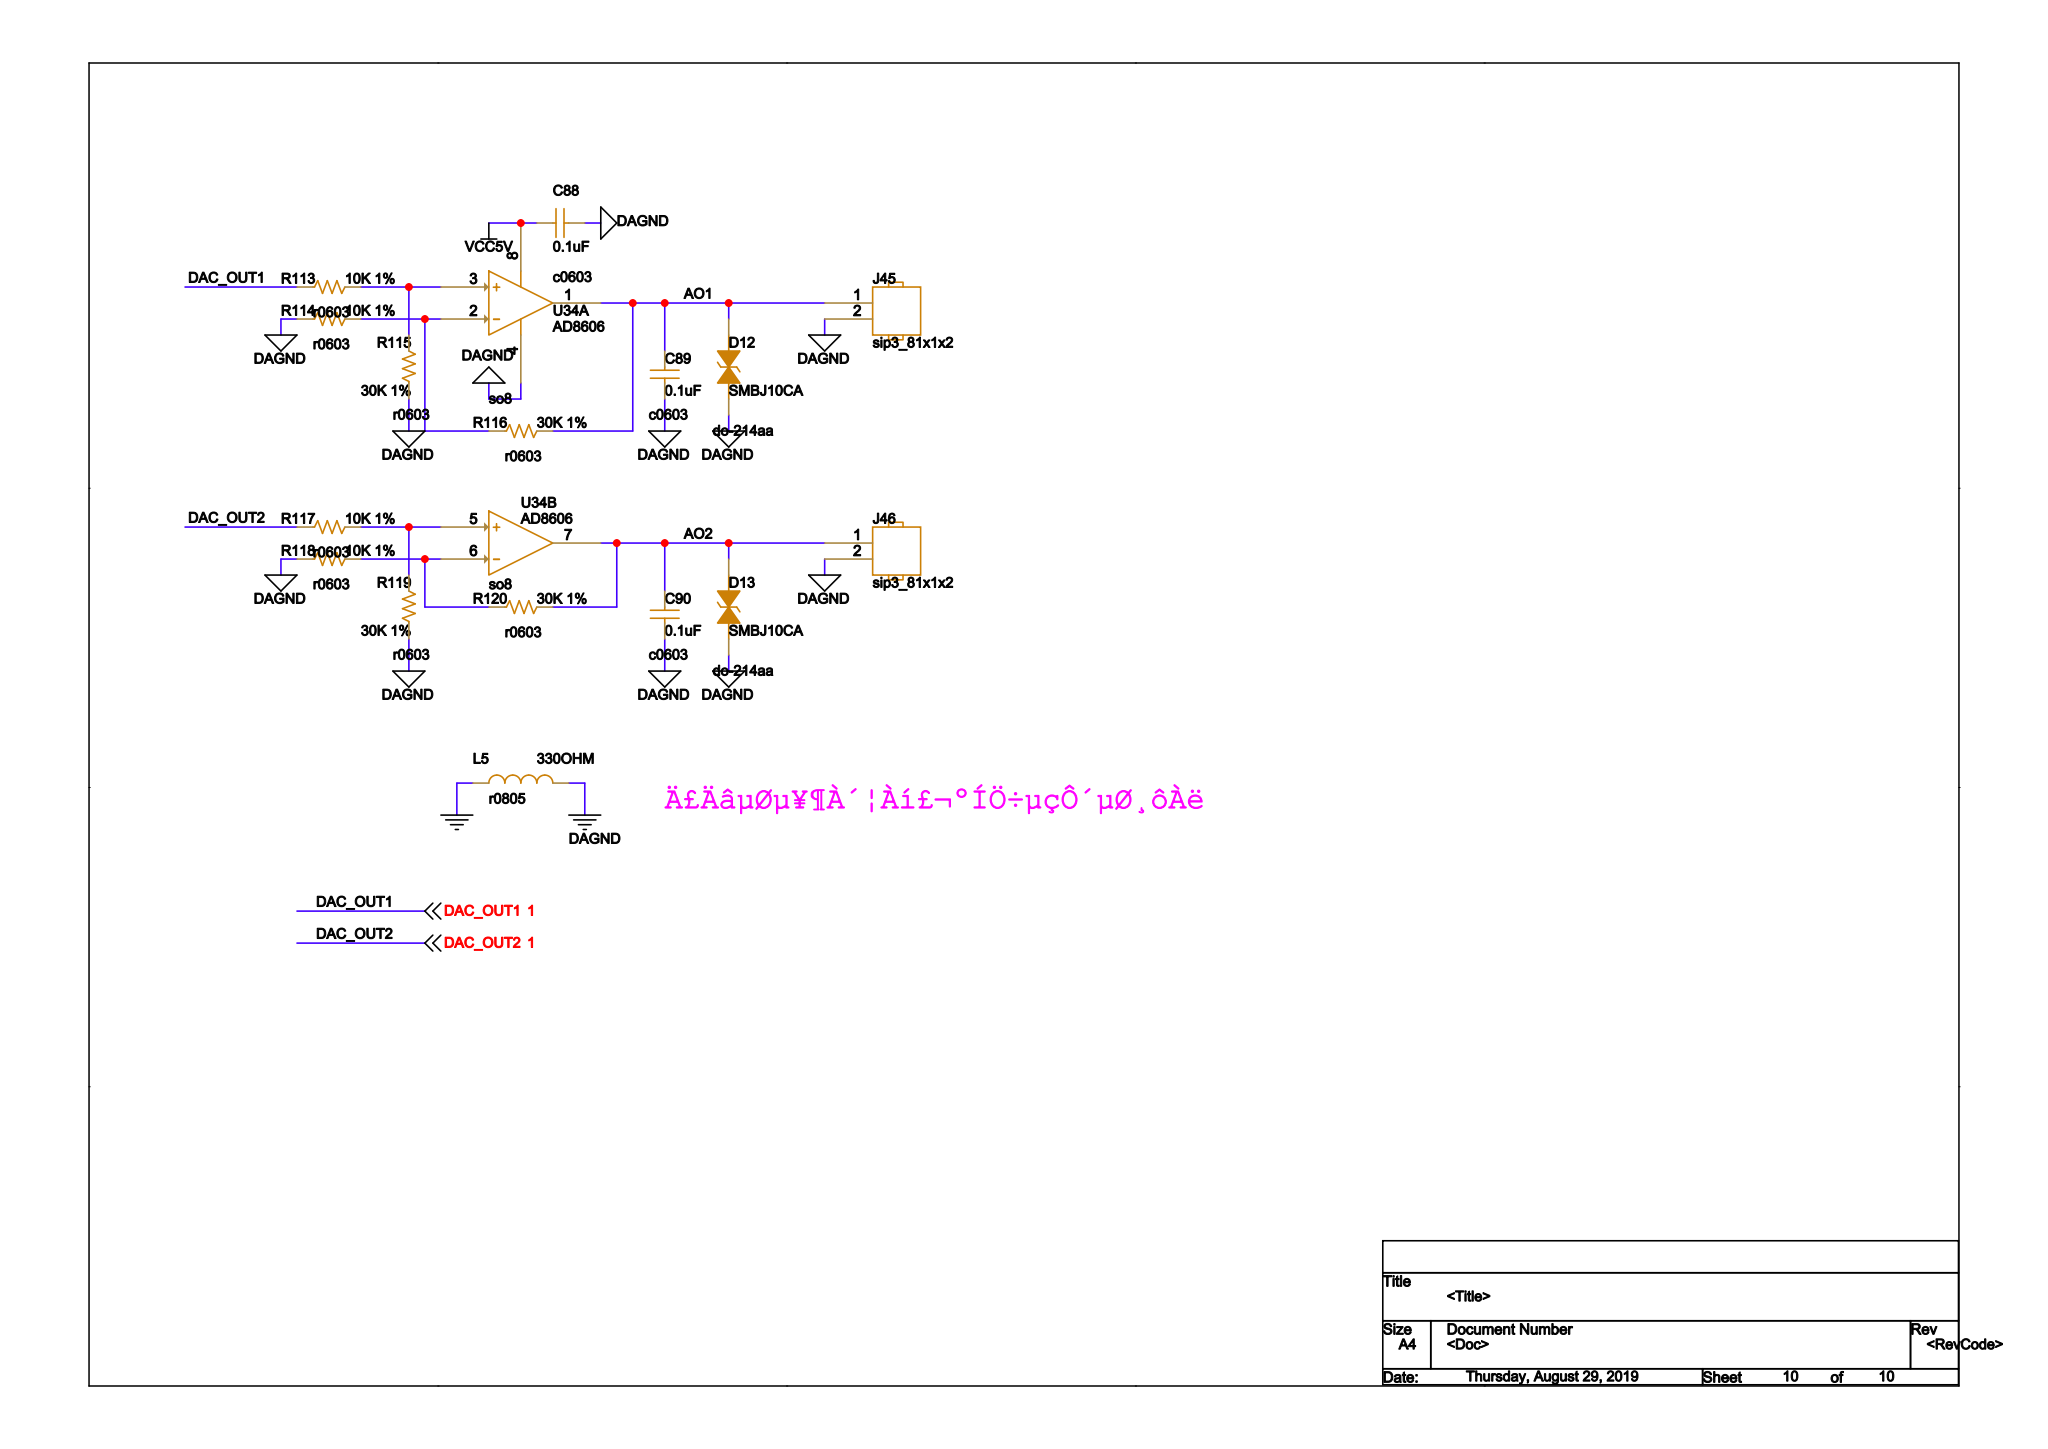Circuit board | Cadence Allegro | 380 parts | 375 nets | one sheet of the schematic
Parts on this sheet (reference | value | footprint):
C88 | 0.1uF | C0603
C89 | 0.1uF | C0603
C90 | 0.1uF | C0603
D12 | SMBJ10CA | DO-214AA
D13 | SMBJ10CA | DO-214AA
J45 | HEADER 2 | SIP3_81X1X2
J46 | HEADER 2 | SIP3_81X1X2
L5 | 330OHM | R0805
R113 | 10K 1% | R0603
R114 | 10K 1% | R0603
R115 | 30K 1% | R0603
R116 | 30K 1% | R0603
R117 | 10K 1% | R0603
R118 | 10K 1% | R0603
R119 | 30K 1% | R0603
R120 | 30K 1% | R0603
Nets of these parts (net: part-pin ...):
GND: L5-1
VCC5V: C88-1
DAGND: C88-2 C89-2 C90-2 D12-1 D13-1 J45-2 J46-2 L5-2 R114-1 R115-1 R118-1 R119-1
AO1: C89-1 D12-2 J45-1 R116-2
AO2: C90-1 D13-2 J46-1 R120-2
DAC_OUT1: R113-1
N1729877: R113-2 R115-2
N1729595: R114-2 R116-1
DAC_OUT2: R117-1
N1730610: R117-2 R119-2
N1730536: R118-2 R120-1